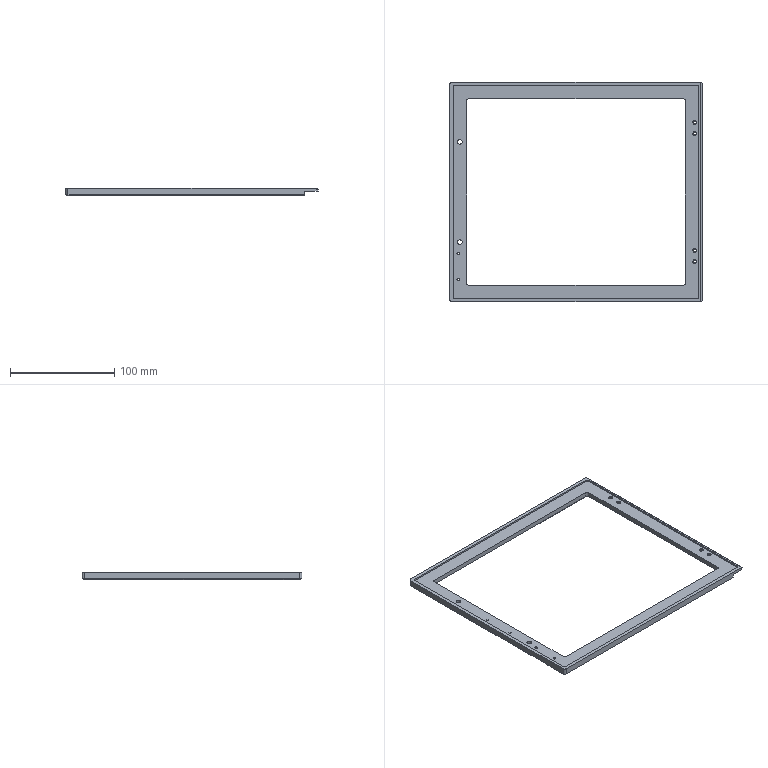NC program | NX | posted with a generic post | part box 241.5 x 210.5 x 7 mm
Whole program:
N10 G17 G21 G94 G90
(FLOOR_WALL_COPY , TOOL : D10)
N12 T10 M6
N14 G54
N16 G17 G0 G90 X128.75 Y-105.247 S9500 M3
N18 G43 Z75. H10
N20 Z5.033
N22 G94 G1 Z2.033 F800.
N24 X125.75
N26 X-125.75 F3000.
N28 Y-97.305
N30 X125.75
N32 Y-89.363
N34 X-125.75
N36 Y-81.42
N38 X-104.75
N40 Y-73.478
N42 X-125.75
N44 Y-65.536
N46 X-104.75
N48 Y-57.594
N50 X-125.75
N52 Y-49.652
N54 X-104.75
N56 Y-41.709
N58 X-125.75
N60 Y-33.767
N62 X-104.75
N64 Y-25.825
N66 X-125.75
N68 Y-17.883
N70 X-104.75
N72 Y-9.941
N74 X-125.75
N76 Y-1.999
N78 X-104.75
N80 Y5.944
N82 X-125.75
N84 Y13.886
N86 X-104.75
N88 Y21.828
N90 X-125.75
N92 Y29.77
N94 X-104.75
N96 Y37.712
N98 X-125.75
N100 Y45.655
N102 X-104.75
N104 Y53.597
N106 X-125.75
N108 Y61.539
N110 X-104.75
N112 Y69.481
N114 X-125.75
N116 Y77.423
N118 X-104.75
N120 Y85.366
N122 X-125.75
N124 X-128.75
N126 Z5.033
N128 G0 Z75.
N130 X104.75 Y-66.617
N132 Z6.
N134 G1 Y-81.42 Z2.033 F800.
N136 X125.75 F3000.
N138 Y-73.478
N140 X104.75
N142 Y-65.536
N144 X125.75
N146 Y-57.594
N148 X104.75
N150 Y-49.652
N152 X125.75
N154 Y-41.709
N156 X104.75
N158 Y-33.767
N160 X125.75
N162 Y-25.825
N164 X104.75
N166 Y-17.883
N168 X125.75
N170 Y-9.941
N172 X104.75
N174 Y-1.999
N176 X125.75
N178 Y5.944
N180 X104.75
N182 Y13.886
N184 X125.75
N186 Y21.828
N188 X104.75
N190 Y29.77
N192 X125.75
N194 Y37.712
N196 X104.75
N198 Y45.655
N200 X125.75
N202 Y53.597
N204 X104.75
N206 Y61.539
N208 X125.75
N210 Y69.481
N212 X104.75
N214 Y77.423
N216 X125.75
N218 Y85.366
N220 X104.75
N222 X101.75
N224 Z5.033
N226 G0 Z75.
N228 X-128.75 Y93.308
N230 Z5.033
N232 G1 Z2.033 F800.
N234 X-125.75
N236 X125.75 F3000.
N238 Y101.25
N240 X-125.75
N242 X-128.75
N244 Z5.033
N246 G0 Z75.
N248 X128.75 Y-105.247
N250 Z4.067
N252 G1 Z1.067 F800.
N254 X125.75
N256 X-125.75 F3000.
N258 Y-97.305
N260 X125.75
N262 Y-89.363
N264 X-125.75
N266 Y-81.42
N268 X-104.75
N270 Y-73.478
N272 X-125.75
N274 Y-65.536
N276 X-104.75
N278 Y-57.594
N280 X-125.75
N282 Y-49.652
N284 X-104.75
N286 Y-41.709
N288 X-125.75
N290 Y-33.767
N292 X-104.75
N294 Y-25.825
N296 X-125.75
N298 Y-17.883
N300 X-104.75
N302 Y-9.941
N304 X-125.75
N306 Y-1.999
N308 X-104.75
N310 Y5.944
N312 X-125.75
N314 Y13.886
N316 X-104.75
N318 Y21.828
N320 X-125.75
N322 Y29.77
N324 X-104.75
N326 Y37.712
N328 X-125.75
N330 Y45.655
N332 X-104.75
N334 Y53.597
N336 X-125.75
N338 Y61.539
N340 X-104.75
N342 Y69.481
N344 X-125.75
N346 Y77.423
N348 X-104.75
N350 Y85.366
N352 X-125.75
N354 X-128.75
N356 Z4.067
N358 G0 Z75.
N360 X104.75 Y-66.617
N362 Z5.033
N364 G1 Y-81.42 Z1.067 F800.
N366 X125.75 F3000.
N368 Y-73.478
N370 X104.75
N372 Y-65.536
N374 X125.75
N376 Y-57.594
N378 X104.75
N380 Y-49.652
N382 X125.75
N384 Y-41.709
N386 X104.75
N388 Y-33.767
N390 X125.75
N392 Y-25.825
N394 X104.75
N396 Y-17.883
N398 X125.75
N400 Y-9.941
N402 X104.75
N404 Y-1.999
N406 X125.75
N408 Y5.944
N410 X104.75
N412 Y13.886
N414 X125.75
N416 Y21.828
N418 X104.75
N420 Y29.77
N422 X125.75
N424 Y37.712
N426 X104.75
N428 Y45.655
N430 X125.75
N432 Y53.597
N434 X104.75
N436 Y61.539
N438 X125.75
N440 Y69.481
N442 X104.75
N444 Y77.423
N446 X125.75
N448 Y85.366
N450 X104.75
N452 X101.75
N454 Z4.067
N456 G0 Z75.
N458 X-128.75 Y93.308
N460 Z4.067
N462 G1 Z1.067 F800.
N464 X-125.75
N466 X125.75 F3000.
N468 Y101.25
N470 X-125.75
N472 X-128.75
N474 Z4.067
N476 G0 Z75.
N478 X128.75 Y-105.247
N480 Z3.1
N482 G1 Z0.1 F800.
N484 X125.75
N486 X-125.75 F3000.
N488 Y-97.305
N490 X125.75
N492 Y-89.363
N494 X-125.75
N496 Y-81.42
N498 X-104.75
N500 Y-73.478
N502 X-125.75
N504 Y-65.536
N506 X-104.75
N508 Y-57.594
N510 X-125.75
N512 Y-49.652
N514 X-104.75
N516 Y-41.709
N518 X-125.75
N520 Y-33.767
N522 X-104.75
N524 Y-25.825
N526 X-125.75
N528 Y-17.883
N530 X-104.75
N532 Y-9.941
N534 X-125.75
N536 Y-1.999
N538 X-104.75
N540 Y5.944
N542 X-125.75
N544 Y13.886
N546 X-104.75
N548 Y21.828
N550 X-125.75
N552 Y29.77
N554 X-104.75
N556 Y37.712
N558 X-125.75
N560 Y45.655
N562 X-104.75
N564 Y53.597
N566 X-125.75
N568 Y61.539
N570 X-104.75
N572 Y69.481
N574 X-125.75
N576 Y77.423
N578 X-104.75
N580 Y85.366
N582 X-125.75
N584 X-128.75
N586 Z3.1
N588 G0 Z75.
N590 X104.75 Y-66.617
N592 Z4.067
N594 G1 Y-81.42 Z0.1 F800.
N596 X125.75 F3000.
N598 Y-73.478
N600 X104.75
N602 Y-65.536
N604 X125.75
N606 Y-57.594
N608 X104.75
N610 Y-49.652
N612 X125.75
N614 Y-41.709
N616 X104.75
N618 Y-33.767
N620 X125.75
N622 Y-25.825
N624 X104.75
N626 Y-17.883
N628 X125.75
N630 Y-9.941
N632 X104.75
N634 Y-1.999
N636 X125.75
N638 Y5.944
N640 X104.75
N642 Y13.886
N644 X125.75
N646 Y21.828
N648 X104.75
N650 Y29.77
N652 X125.75
N654 Y37.712
N656 X104.75
N658 Y45.655
N660 X125.75
N662 Y53.597
N664 X104.75
N666 Y61.539
N668 X125.75
N670 Y69.481
N672 X104.75
N674 Y77.423
N676 X125.75
N678 Y85.366
N680 X104.75
N682 X101.75
N684 Z3.1
N686 G0 Z75.
N688 X-128.75 Y93.308
N690 Z3.1
N692 G1 Z0.1 F800.
N694 X-125.75
N696 X125.75 F3000.
N698 Y101.25
N700 X-125.75
N702 X-128.75
N704 Z3.1
N706 G0 Z75.
(FLOOR_WALL_COPY_COPY , TOOL : D10)
N708 X128.75 Y-105.247
N710 Z3.
N712 G1 Z0. F800.
N714 X125.75
N716 X-125.75 F1400.
N718 Y-97.305
N720 X125.75
N722 Y-89.363
N724 X-125.75
N726 Y-81.42
N728 X-104.75
N730 Y-73.478
N732 X-125.75
N734 Y-65.536
N736 X-104.75
N738 Y-57.594
N740 X-125.75
N742 Y-49.652
N744 X-104.75
N746 Y-41.709
N748 X-125.75
N750 Y-33.767
N752 X-104.75
N754 Y-25.825
N756 X-125.75
N758 Y-17.883
N760 X-104.75
N762 Y-9.941
N764 X-125.75
N766 Y-1.999
N768 X-104.75
N770 Y5.944
N772 X-125.75
N774 Y13.886
N776 X-104.75
N778 Y21.828
N780 X-125.75
N782 Y29.77
N784 X-104.75
N786 Y37.712
N788 X-125.75
N790 Y45.655
N792 X-104.75
N794 Y53.597
N796 X-125.75
N798 Y61.539
N800 X-104.75
N802 Y69.481
N804 X-125.75
N806 Y77.423
N808 X-104.75
N810 Y85.366
N812 X-125.75
N814 X-128.75
N816 Z3.
N818 G0 Z75.
N820 X104.75 Y-59.029
N822 Z6.
N824 G1 Y-81.42 Z0. F800.
N826 X125.75 F1400.
N828 Y-73.478
N830 X104.75
N832 Y-65.536
N834 X125.75
N836 Y-57.594
N838 X104.75
N840 Y-49.652
N842 X125.75
N844 Y-41.709
N846 X104.75
N848 Y-33.767
N850 X125.75
N852 Y-25.825
N854 X104.75
N856 Y-17.883
N858 X125.75
N860 Y-9.941
N862 X104.75
N864 Y-1.999
N866 X125.75
N868 Y5.944
N870 X104.75
N872 Y13.886
N874 X125.75
N876 Y21.828
N878 X104.75
N880 Y29.77
N882 X125.75
N884 Y37.712
N886 X104.75
N888 Y45.655
N890 X125.75
N892 Y53.597
N894 X104.75
N896 Y61.539
N898 X125.75
N900 Y69.481
N902 X104.75
N904 Y77.423
N906 X125.75
N908 Y85.366
N910 X104.75
N912 X101.75
N914 Z3.
N916 G0 Z75.
N918 X-128.75 Y93.308
N920 Z3.
N922 G1 Z0. F800.
N924 X-125.75
N926 X125.75 F1400.
N928 Y101.25
N930 X-125.75
N932 X-128.75
N934 Z3.
N936 G0 Z75.
N938 M5
(FLOOR_WALL_2 , TOOL : D6)
N940 T06 M6
N942 G54
N944 G17 G0 G90 X-114.75 Y73.689 S9500 M3
N946 G43 Z75. H6
N948 Z1.1
N950 G94 G1 Y68.092 Z0.807 F1000.
N952 X-114.194 Y67.604 Z0.768
N954 X-113.102 Y66.237 Z0.676
N956 X-112.75 Y65.587 Z0.637
N958 X-112.398 Y66.237 Z0.599
N960 X-111.306 Y67.604 Z0.507
N962 X-110.75 Y68.092 Z0.468
N964 Y74.408 Z0.137
N966 X-111.306 Y74.896 Z0.098
N968 X-112.398 Y76.263 Z0.007
N970 X-112.75 Y76.913 Z-0.032
N972 X-113.102 Y76.263 Z-0.071
N974 X-114.194 Y74.896 Z-0.162
N976 X-114.75 Y74.408 Z-0.201
N978 Y71.25 Z-0.367
N980 Y68.092 F2500.
N982 G2 X-112.75 Y65.587 R9.1
N984 X-110.75 Y68.092 R9.1
N986 G1 Y74.408
N988 G2 X-112.75 Y76.913 R9.1
N990 X-114.75 Y74.408 R9.1
N992 G1 Y71.25
N994 X-117.75
N996 Y66.561
N998 G2 X-114.65 Y61.25 R6.1
N1000 G3 X-112.75 Y59.35 R1.9
N1002 X-110.85 Y61.25 R1.9
N1004 G2 X-107.75 Y66.561 R6.1
N1006 G1 Y75.939
N1008 G2 X-110.85 Y81.25 R6.1
N1010 G3 X-112.75 Y83.15 R1.9
N1012 X-114.65 Y81.25 R1.9
N1014 G2 X-117.75 Y75.939 R6.1
N1016 G1 Y71.25
N1018 X-120.75
N1020 Y64.35
N1022 G2 X-117.65 Y61.25 R3.1
N1024 G3 X-112.75 Y56.35 R4.9
N1026 X-107.85 Y61.25 R4.9
N1028 G2 X-104.75 Y64.35 R3.1
N1030 G1 Y78.15
N1032 G2 X-107.85 Y81.25 R3.1
N1034 G3 X-112.75 Y86.15 R4.9
N1036 X-117.65 Y81.25 R4.9
N1038 G2 X-120.75 Y78.15 R3.1
N1040 G1 Y71.25
N1042 Z0.633
N1044 G0 X-114.75 Y73.689
N1046 G1 Y68.092 Z0.34 F1000.
N1048 X-114.194 Y67.604 Z0.301
N1050 X-113.102 Y66.237 Z0.21
N1052 X-112.75 Y65.587 Z0.171
N1054 X-112.398 Y66.237 Z0.132
N1056 X-111.306 Y67.604 Z0.04
N1058 X-110.75 Y68.092 Z0.002
N1060 Y74.408 Z-0.329
N1062 X-111.306 Y74.896 Z-0.368
N1064 X-112.398 Y76.263 Z-0.46
N1066 X-112.75 Y76.913 Z-0.499
N1068 X-113.102 Y76.263 Z-0.537
N1070 X-114.194 Y74.896 Z-0.629
N1072 X-114.75 Y74.408 Z-0.668
N1074 Y71.25 Z-0.833
N1076 Y68.092 F2500.
N1078 G2 X-112.75 Y65.587 R9.1
N1080 X-110.75 Y68.092 R9.1
N1082 G1 Y74.408
N1084 G2 X-112.75 Y76.913 R9.1
N1086 X-114.75 Y74.408 R9.1
N1088 G1 Y71.25
N1090 X-117.75
N1092 Y66.561
N1094 G2 X-114.65 Y61.25 R6.1
N1096 G3 X-112.75 Y59.35 R1.9
N1098 X-110.85 Y61.25 R1.9
N1100 G2 X-107.75 Y66.561 R6.1
N1102 G1 Y75.939
N1104 G2 X-110.85 Y81.25 R6.1
N1106 G3 X-112.75 Y83.15 R1.9
N1108 X-114.65 Y81.25 R1.9
N1110 G2 X-117.75 Y75.939 R6.1
N1112 G1 Y71.25
N1114 X-120.75
N1116 Y64.35
N1118 G2 X-117.65 Y61.25 R3.1
N1120 G3 X-112.75 Y56.35 R4.9
N1122 X-107.85 Y61.25 R4.9
N1124 G2 X-104.75 Y64.35 R3.1
N1126 G1 Y78.15
N1128 G2 X-107.85 Y81.25 R3.1
N1130 G3 X-112.75 Y86.15 R4.9
N1132 X-117.65 Y81.25 R4.9
N1134 G2 X-120.75 Y78.15 R3.1
N1136 G1 Y71.25
N1138 Z0.167
N1140 G0 X-114.75 Y73.689
N1142 G1 Y68.092 Z-0.127 F1000.
N1144 X-114.194 Y67.604 Z-0.165
N1146 X-113.102 Y66.237 Z-0.257
N1148 X-112.75 Y65.587 Z-0.296
N1150 X-112.398 Y66.237 Z-0.335
N1152 X-111.306 Y67.604 Z-0.426
N1154 X-110.75 Y68.092 Z-0.465
N1156 Y74.408 Z-0.796
N1158 X-111.306 Y74.896 Z-0.835
N1160 X-112.398 Y76.263 Z-0.927
N1162 X-112.75 Y76.913 Z-0.965
N1164 X-113.102 Y76.263 Z-1.004
N1166 X-114.194 Y74.896 Z-1.096
N1168 X-114.75 Y74.408 Z-1.134
N1170 Y71.25 Z-1.3
N1172 Y68.092 F2500.
N1174 G2 X-112.75 Y65.587 R9.1
N1176 X-110.75 Y68.092 R9.1
N1178 G1 Y74.408
N1180 G2 X-112.75 Y76.913 R9.1
N1182 X-114.75 Y74.408 R9.1
N1184 G1 Y71.25
N1186 X-117.75
N1188 Y66.561
N1190 G2 X-114.65 Y61.25 R6.1
N1192 G3 X-112.75 Y59.35 R1.9
N1194 X-110.85 Y61.25 R1.9
N1196 G2 X-107.75 Y66.561 R6.1
N1198 G1 Y75.939
N1200 G2 X-110.85 Y81.25 R6.1
N1202 G3 X-112.75 Y83.15 R1.9
N1204 X-114.65 Y81.25 R1.9
N1206 G2 X-117.75 Y75.939 R6.1
N1208 G1 Y71.25
N1210 X-120.75
N1212 Y64.35
N1214 G2 X-117.65 Y61.25 R3.1
N1216 G3 X-112.75 Y56.35 R4.9
N1218 X-107.85 Y61.25 R4.9
N1220 G2 X-104.75 Y64.35 R3.1
N1222 G1 Y78.15
N1224 G2 X-107.85 Y81.25 R3.1
N1226 G3 X-112.75 Y86.15 R4.9
N1228 X-117.65 Y81.25 R4.9
N1230 G2 X-120.75 Y78.15 R3.1
N1232 G1 Y71.25
N1234 Z-0.3
N1236 G0 Z75.
N1238 X-111.85 Y16.614
N1240 Z1.
N1242 G1 Y25.4 Z0.54 F1000.
N1244 X-113.65 Z0.445
N1246 Y8. Z-0.467
N1248 Y-9.4 F2500.
N1250 X-111.85
N1252 Y25.4
N1254 X-113.65
N1256 Y8.
N1258 X-116.65
N1260 Y-12.4
N1262 X-108.85
N1264 Y28.4
N1266 X-116.65
N1268 Y8.
N1270 Z0.533
N1272 G0 X-111.85 Y16.614
N1274 G1 Y25.4 Z0.073 F1000.
N1276 X-113.65 Z-0.021
N1278 Y8. Z-0.933
N1280 Y-9.4 F2500.
N1282 X-111.85
N1284 Y25.4
N1286 X-113.65
N1288 Y8.
N1290 X-116.65
N1292 Y-12.4
N1294 X-108.85
N1296 Y28.4
N1298 X-116.65
N1300 Y8.
N1302 Z0.067
N1304 G0 X-111.85 Y16.614
N1306 G1 Y25.4 Z-0.394 F1000.
N1308 X-113.65 Z-0.488
N1310 Y8. Z-1.4
N1312 Y-9.4 F2500.
N1314 X-111.85
N1316 Y25.4
N1318 X-113.65
N1320 Y8.
N1322 X-116.65
N1324 Y-12.4
N1326 X-108.85
N1328 Y28.4
N1330 X-116.65
N1332 Y8.
N1334 Z-0.4
N1336 G0 Z75.
(FLOOR_WALL_4 , TOOL : D6)
N1338 X-109.053 Y24.095
N1340 Z-0.4
N1342 G1 Y28.2 Z-1.5 F1250.
N1344 Y-12.2
N1346 X-111.519
N1348 Y28.2
N1350 X-113.984
N1352 Y-12.2
N1354 X-116.45
N1356 Y28.2
N1358 Y27.5
N1360 Y28.5
N1362 X-116.75
N1364 Y-12.5
N1366 X-108.75
N1368 Y28.5
N1370 X-116.45
N1372 Y27.5
N1374 X-115.75
N1376 Z-0.5
N1378 G0 Z75.
N1380 X120.747 Y108.908
N1382 Z-3.4
N1384 G1 Z-4.4
N1386 Y107.834
N1388 Y-107.834
N1390 G2 X118.75 Y-108.25 R5.
N1392 G1 X118.29
N1394 Y108.25
N1396 X115.833
N1398 Y-108.25
N1400 X113.376
N1402 Y108.25
N1404 X111.05
N1406 Y73.15
N1408 G2 X110.918 Y72.227 R3.3
N1410 G1 Z-3.4
N1412 G0 Z75.
N1414 Z-3.4
N1416 G1 Z-4.4
N1418 G2 X111.099 Y71.151 R3.3
N1420 G1 Y51.849
N1422 G2 X110.918 Y50.773 R3.3
N1424 G1 Z-3.4
N1426 G0 Z75.
N1428 Z-3.4
N1430 G1 Z-4.4
N1432 G2 X111.05 Y49.85 R3.3
N1434 G1 Y-49.85
N1436 G2 X110.918 Y-50.773 R3.3
N1438 G1 Z-3.4
N1440 G0 Z75.
N1442 Z-3.4
N1444 G1 Z-4.4
N1446 G2 X111.099 Y-51.849 R3.3
N1448 G1 Y-71.151
N1450 G2 X110.918 Y-72.227 R3.3
N1452 G1 Z-3.4
N1454 G0 Z75.
N1456 X110.75 Y109.25
N1458 Z-3.4
N1460 G1 Z-4.4
N1462 Y108.25
N1464 Y73.15
N1466 G2 X110.602 Y72.219 R3.
N1468 X110.799 Y71.151 R3.
N1470 G1 Y51.849
N1472 G2 X110.602 Y50.781 R3.
N1474 X110.75 Y49.85 R3.
N1476 G1 Y-49.85
N1478 G2 X110.602 Y-50.781 R3.
N1480 X110.799 Y-51.849 R3.
N1482 G1 Y-71.151
N1484 G2 X110.602 Y-72.219 R3.
N1486 X110.75 Y-73.15 R3.
N1488 G1 Y-108.25
N1490 Y-109.25
N1492 Z-3.4
N1494 G0 Z75.
(FLOOR_WALL_4_COPY , TOOL : D6)
N1496 X-113.88 Y74.98
N1498 Z-0.3
N1500 G1 X-114.179 Y74.627 Z-0.424
N1502 X-114.75 Y74.144 Z-0.624
N1504 Y71.25 Z-1.4
N1506 Y68.356
N1508 G2 X-112.75 Y65.992 R9.3
N1510 X-110.75 Y68.356 R9.3
N1512 G1 Y74.144
N1514 G2 X-112.75 Y76.508 R9.3
N1516 X-114.75 Y74.144 R9.3
N1518 G1 Y71.25
N1520 X-117.75
N1522 Y66.79
N1524 G2 X-114.45 Y61.25 R6.3
N1526 G3 X-112.75 Y59.55 R1.7
N1528 X-111.05 Y61.25 R1.7
N1530 G2 X-107.75 Y66.79 R6.3
N1532 G1 Y75.71
N1534 G2 X-111.05 Y81.25 R6.3
N1536 G3 X-112.75 Y82.95 R1.7
N1538 X-114.45 Y81.25 R1.7
N1540 G2 X-117.75 Y75.71 R6.3
N1542 G1 Y71.25
N1544 X-120.75
N1546 Y64.55
N1548 G2 X-117.45 Y61.25 R3.3
N1550 G3 X-112.75 Y56.55 R4.7
N1552 X-108.05 Y61.25 R4.7
N1554 G2 X-104.75 Y64.55 R3.3
N1556 G1 Y77.95
N1558 G2 X-108.05 Y81.25 R3.3
N1560 G3 X-112.75 Y85.95 R4.7
N1562 X-117.45 Y81.25 R4.7
N1564 G2 X-120.75 Y77.95 R3.3
N1566 G1 Y71.25
N1568 G2 X-121.05 Y70.73 R0.6
N1570 G1 X-123.87
N1572 Z-0.4
N1574 G0 Z75.
N1576 X-120.63 Y64.668
N1578 Z-0.4
N1580 G1 Z-1.4
N1582 X-121.27 Y64.55
N1584 G3 X-120.75 Y64.25 R0.6
N1586 G2 X-117.75 Y61.25 R3.
N1588 G3 X-112.75 Y56.25 R5.
N1590 X-107.75 Y61.25 R5.
N1592 G2 X-104.75 Y64.25 R3.
N1594 G3 X-104.23 Y64.55 R0.6
N1596 G1 X-104.87 Y64.668
N1598 Z-0.4
N1600 G0 Z75.
N1602 Y77.832
N1604 Z-0.4
N1606 G1 Z-1.4
N1608 X-104.23 Y77.95
N1610 G3 X-104.75 Y78.25 R0.6
N1612 G2 X-107.75 Y81.25 R3.
N1614 G3 X-112.75 Y86.25 R5.
N1616 X-117.75 Y81.25 R5.
N1618 G2 X-120.75 Y78.25 R3.
N1620 G3 X-121.27 Y77.95 R0.6
N1622 G1 X-120.63 Y77.832
N1624 Z-0.4
N1626 G0 Z75.
N1628 M5
(CAVITY_MILL_COPY , TOOL : D2)
N1630 T02 M6
N1632 G54
N1634 G17 G0 G90 X109.199 Y-70.396 S9500 M3
N1636 G43 Z75. H2
N1638 Z-0.13
N1640 G94 G3 X108.797 Y-71.175 R1. F1000.
N1642 G1 Y-71.183 F1100.
N1644 G2 X108.306 Y-72.011 R0.995
N1646 X107.907 Y-72.162 R1.295
N1648 G1 X107.949 Y-72.17
N1650 G2 X108.75 Y-73.175 R1.
N1652 G3 X109.15 Y-73.975 R1.
N1654 G0 X109.199 Y-70.396 Z-0.326
N1656 G3 X108.797 Y-71.175 R1. F1000.
N1658 G1 Y-71.182 F1100.
N1660 G2 X108.306 Y-72.011 R0.995
N1662 X107.907 Y-72.162 R1.297
N1664 G1 X107.91 Y-72.164
N1666 X107.949 Y-72.17
N1668 G2 X108.75 Y-73.175 R1.
N1670 G3 X109.15 Y-73.975 R1.
N1672 G0 X109.199 Y-70.396 Z-0.522
N1674 G3 X108.797 Y-71.175 R1. F1000.
N1676 G1 Y-71.181 F1100.
N1678 G2 X108.306 Y-72.011 R0.995
N1680 X107.907 Y-72.162 R1.298
N1682 G1 X107.948 Y-72.17
N1684 G2 X108.75 Y-73.175 R1.
N1686 G3 X109.15 Y-73.975 R1.
N1688 G0 X109.199 Y-70.395 Z-0.717
N1690 G3 X108.797 Y-71.175 R1. F1000.
N1692 G1 Y-71.18 F1100.
N1694 G2 X108.306 Y-72.012 R0.995
N1696 X107.907 Y-72.162 R1.3
N1698 G1 X107.947 Y-72.17
N1700 G2 X108.75 Y-73.175 R1.
N1702 G3 X109.15 Y-73.975 R1.
N1704 G0 X109.199 Y-70.395 Z-0.913
N1706 G3 X108.797 Y-71.175 R1. F1000.
N1708 G1 Y-71.179 F1100.
N1710 G2 X108.306 Y-72.012 R0.995
N1712 X107.907 Y-72.162 R1.302
N1714 G1 X107.947 Y-72.17
N1716 G2 X108.75 Y-73.175 R1.
N1718 G3 X109.15 Y-73.975 R1.
N1720 G0 X109.199 Y-70.395 Z-1.109
N1722 G3 X108.797 Y-71.175 R1. F1000.
N1724 G1 Y-71.179 F1100.
N1726 G2 X108.306 Y-72.012 R0.995
N1728 X107.907 Y-72.162 R1.303
N1730 G1 X107.946 Y-72.169
N1732 G2 X108.75 Y-73.175 R1.
N1734 G3 X109.15 Y-73.975 R1.
N1736 G0 X109.199 Y-70.395 Z-1.304
N1738 G3 X108.797 Y-71.175 R1. F1000.
N1740 G1 Y-71.178 F1100.
N1742 G2 X108.306 Y-72.012 R0.995
N1744 X107.907 Y-72.162 R1.305
N1746 G1 X107.945 Y-72.169
N1748 G2 X108.75 Y-73.175 R1.
N1750 G3 X109.15 Y-73.975 R1.
N1752 G0 X109.199 Y-70.395 Z-1.5
N1754 G3 X108.797 Y-71.175 R1. F1000.
N1756 G1 Y-71.177 F1100.
N1758 G2 X108.306 Y-72.012 R0.994
N1760 X107.907 Y-72.162 R1.307
N1762 G1 X107.945 Y-72.169
N1764 G2 X108.75 Y-73.175 R1.
N1766 G3 X109.15 Y-73.975 R1.
N1768 G0 X109.199 Y-70.394 Z-1.693
N1770 G3 X108.797 Y-71.175 R1. F1000.
N1772 G2 X108.306 Y-72.012 R0.994 F1100.
N1774 X107.907 Y-72.162 R1.308
N1776 G1 X107.944 Y-72.169
N1778 G2 X108.75 Y-73.175 R1.
N1780 G3 X109.15 Y-73.975 R1.
N1782 G0 X109.199 Y-70.394 Z-1.887
N1784 G3 X108.797 Y-71.175 R1. F1000.
N1786 G2 X108.306 Y-72.012 R0.994 F1100.
N1788 X107.907 Y-72.162 R1.31
N1790 G1 X107.943 Y-72.169
N1792 G2 X108.75 Y-73.175 R1.
N1794 G3 X109.15 Y-73.975 R1.
N1796 G0 X109.199 Y-70.394 Z-2.08
N1798 G3 X108.797 Y-71.175 R1. F1000.
N1800 G2 X108.306 Y-72.012 R0.993 F1100.
N1802 X107.907 Y-72.162 R1.312
N1804 G1 X107.942 Y-72.169
N1806 G2 X108.75 Y-73.175 R1.
N1808 G3 X109.15 Y-73.975 R1.
N1810 G0 X109.199 Y-70.396 Z-2.273
N1812 G3 X108.797 Y-71.175 R1. F1000.
N1814 G2 X108.306 Y-72.012 R0.996 F1100.
N1816 X107.907 Y-72.162 R1.313
N1818 G1 X107.941 Y-72.168
N1820 G2 X108.75 Y-73.176 R1.
N1822 G3 X109.15 Y-73.976 R1.
N1824 G0 X109.199 Y-70.396 Z-2.467
N1826 G3 X108.798 Y-71.175 R1. F1000.
N1828 G2 X108.306 Y-72.012 R0.997 F1100.
N1830 X107.907 Y-72.162 R1.315
N1832 G1 X107.941 Y-72.168
N1834 G2 X108.75 Y-73.176 R1.
N1836 G3 X109.15 Y-73.976 R1.
N1838 G0 X109.199 Y-70.396 Z-2.66
N1840 G3 X108.798 Y-71.175 R1. F1000.
N1842 G2 X108.306 Y-72.012 R0.997 F1100.
N1844 X107.907 Y-72.162 R1.317
N1846 G1 X107.94 Y-72.168
N1848 G2 X108.75 Y-73.176 R1.
N1850 G3 X109.15 Y-73.976 R1.
N1852 G0 X109.199 Y-70.397 Z-2.853
N1854 G3 X108.798 Y-71.175 R1. F1000.
N1856 G2 X108.306 Y-72.013 R0.998 F1100.
N1858 X107.907 Y-72.162 R1.318
N1860 G1 X107.939 Y-72.168
N1862 G2 X108.75 Y-73.176 R1.
N1864 G3 X109.15 Y-73.976 R1.
N1866 G0 X109.199 Y-70.397 Z-3.047
N1868 G3 X108.798 Y-71.175 R1. F1000.
N1870 G2 X108.306 Y-72.013 R0.998 F1100.
N1872 X107.907 Y-72.162 R1.32
N1874 G1 X107.938 Y-72.168
N1876 G2 X108.75 Y-73.176 R1.
N1878 G3 X109.15 Y-73.976 R1.
N1880 G0 X109.199 Y-70.397 Z-3.24
N1882 G3 X108.798 Y-71.175 R1. F1000.
N1884 G2 X108.306 Y-72.013 R0.998 F1100.
N1886 X107.907 Y-72.162 R1.322
N1888 G1 X107.936 Y-72.168
N1890 G2 X108.75 Y-73.176 R1.
N1892 G3 X109.15 Y-73.976 R1.
N1894 G0 X109.199 Y-70.398 Z-3.433
N1896 G3 X108.798 Y-71.175 R1. F1000.
N1898 G2 X108.306 Y-72.013 R0.999 F1100.
N1900 X107.907 Y-72.162 R1.324
N1902 G1 X107.935 Y-72.167
N1904 G2 X108.75 Y-73.176 R1.
N1906 G3 X109.15 Y-73.976 R1.
N1908 G0 X109.199 Y-70.398 Z-3.627
N1910 G3 X108.798 Y-71.175 R1. F1000.
N1912 G2 X108.306 Y-72.013 R0.999 F1100.
N1914 X107.907 Y-72.162 R1.325
N1916 G1 X107.934 Y-72.167
N1918 G2 X108.75 Y-73.176 R1.
N1920 G3 X109.15 Y-73.976 R1.
N1922 G0 X109.199 Y-70.398 Z-3.82
N1924 G3 X108.798 Y-71.175 R1. F1000.
N1926 G2 X108.306 Y-72.013 R0.999 F1100.
N1928 X107.907 Y-72.162 R1.327
N1930 G1 X107.932 Y-72.167
N1932 G2 X108.75 Y-73.176 R1.
N1934 G3 X109.15 Y-73.976 R1.
N1936 G0 X109.199 Y-70.398 Z-4.013
N1938 G3 X108.798 Y-71.175 R1. F1000.
N1940 G2 X108.306 Y-72.013 R0.999 F1100.
N1942 X107.907 Y-72.162 R1.329
N1944 G1 X107.93 Y-72.166
N1946 G2 X108.75 Y-73.176 R1.
N1948 G3 X109.15 Y-73.976 R1.
N1950 G0 X109.199 Y-70.398 Z-4.207
N1952 G3 X108.799 Y-71.175 R1. F1000.
N1954 G2 X108.306 Y-72.013 R0.999 F1100.
N1956 X107.91 Y-72.162 R1.331
N1958 G1 X107.93 Y-72.166
N1960 G2 X108.75 Y-73.176 R1.
N1962 G3 X109.15 Y-73.976 R1.
N1964 G0 X109.199 Y-70.398 Z-4.4
N1966 G3 X108.799 Y-71.175 R1. F1000.
N1968 G2 X108.306 Y-72.013 R0.999 F1100.
N1970 X107.91 Y-72.162 R1.333
N1972 G1 X107.93 Y-72.166
N1974 G2 X108.75 Y-73.176 R1.
N1976 G3 X109.15 Y-73.976 R1.
N1978 G0 Z75.
N1980 Y-48.966
N1982 Z-0.13
N1984 G3 X108.75 Y-49.766 R1. F1000.
N1986 G1 Y-49.85 F1100.
N1988 G2 X107.837 Y-50.846 R1.004
N1990 X108.798 Y-51.837 R1.012
N1992 G3 X109.199 Y-52.618 R1.
N1994 G0 X109.15 Y-48.966 Z-0.326
N1996 G3 X108.75 Y-49.766 R1. F1000.
N1998 G1 Y-49.85 F1100.
N2000 G2 X107.837 Y-50.846 R1.004
N2002 X108.798 Y-51.837 R1.011
N2004 G3 X109.199 Y-52.619 R1.
N2006 G0 X109.15 Y-48.966 Z-0.522
N2008 G3 X108.75 Y-49.766 R1. F1000.
N2010 G1 Y-49.85 F1100.
N2012 G2 X107.837 Y-50.846 R1.003
N2014 X108.798 Y-51.837 R1.011
N2016 G3 X109.199 Y-52.619 R1.
N2018 G0 X109.15 Y-48.966 Z-0.717
N2020 G3 X108.75 Y-49.766 R1. F1000.
N2022 G1 Y-49.85 F1100.
N2024 G2 X107.837 Y-50.846 R1.003
N2026 X108.798 Y-51.837 R1.011
N2028 G3 X109.199 Y-52.619 R1.
N2030 G0 X109.15 Y-48.966 Z-0.913
N2032 G3 X108.75 Y-49.766 R1. F1000.
N2034 G1 Y-49.85 F1100.
N2036 G2 X107.837 Y-50.846 R1.003
N2038 X108.798 Y-51.837 R1.011
N2040 G3 X109.199 Y-52.619 R1.
N2042 G0 X109.15 Y-48.966 Z-1.109
N2044 G3 X108.75 Y-49.766 R1. F1000.
N2046 G1 Y-49.85 F1100.
N2048 G2 X107.838 Y-50.846 R1.003
N2050 X108.798 Y-51.837 R1.011
N2052 G3 X109.199 Y-52.62 R1.
N2054 G0 X109.15 Y-48.966 Z-1.304
N2056 G3 X108.75 Y-49.766 R1. F1000.
N2058 G1 Y-49.85 F1100.
N2060 G2 X107.838 Y-50.846 R1.003
N2062 X108.798 Y-51.837 R1.01
N2064 G3 X109.199 Y-52.62 R1.
N2066 G0 X109.15 Y-48.965 Z-1.5
N2068 G3 X108.75 Y-49.765 R1. F1000.
N2070 G1 Y-49.85 F1100.
N2072 G2 X107.838 Y-50.846 R1.002
N2074 X108.799 Y-51.837 R1.01
N2076 G3 X109.199 Y-52.62 R1.
N2078 G0 X109.15 Y-48.965 Z-1.693
N2080 G3 X108.75 Y-49.765 R1. F1000.
N2082 G1 Y-49.85 F1100.
N2084 G2 X107.838 Y-50.846 R1.002
N2086 X108.799 Y-51.837 R1.01
N2088 G3 X109.199 Y-52.621 R1.
N2090 G0 X109.15 Y-48.965 Z-1.887
N2092 G3 X108.75 Y-49.765 R1. F1000.
N2094 G1 Y-49.85 F1100.
N2096 G2 X107.838 Y-50.846 R1.002
N2098 X108.799 Y-51.837 R1.01
N2100 G3 X109.199 Y-52.621 R1.
N2102 G0 X109.15 Y-48.965 Z-2.08
N2104 G3 X108.75 Y-49.765 R1. F1000.
N2106 G1 Y-49.85 F1100.
N2108 G2 X107.838 Y-50.846 R1.002
N2110 X108.799 Y-51.838 R1.009
N2112 G3 X109.199 Y-52.621 R1.
N2114 G0 X109.15 Y-48.965 Z-2.273
N2116 G3 X108.75 Y-49.765 R1. F1000.
N2118 G1 Y-49.85 F1100.
N2120 G2 X107.838 Y-50.846 R1.001
N2122 X108.799 Y-51.838 R1.009
N2124 G3 X109.199 Y-52.621 R1.
N2126 G0 X109.15 Y-48.965 Z-2.467
N2128 G3 X108.75 Y-49.765 R1. F1000.
N2130 G1 Y-49.85 F1100.
N2132 G2 X107.838 Y-50.846 R1.001
N2134 X108.799 Y-51.838 R1.009
N2136 G3 X109.199 Y-52.622 R1.
N2138 G0 X109.15 Y-48.965 Z-2.66
N2140 G3 X108.75 Y-49.765 R1. F1000.
N2142 G1 Y-49.85 F1100.
N2144 G2 X107.838 Y-50.846 R1.001
N2146 X108.799 Y-51.838 R1.009
N2148 G3 X109.199 Y-52.622 R1.
N2150 G0 X109.15 Y-48.965 Z-2.853
N2152 G3 X108.75 Y-49.765 R1. F1000.
N2154 G1 Y-49.85 F1100.
N2156 G2 X107.838 Y-50.846 R1.001
N2158 X108.799 Y-51.838 R1.009
N2160 G3 X109.199 Y-52.622 R1.
N2162 G0 X109.15 Y-48.965 Z-3.047
N2164 G3 X108.75 Y-49.765 R1. F1000.
N2166 G1 Y-49.85 F1100.
N2168 G2 X107.838 Y-50.846 R1.
N2170 X108.799 Y-51.838 R1.008
N2172 G3 X109.199 Y-52.622 R1.
N2174 G0 X109.15 Y-48.965 Z-3.24
N2176 G3 X108.75 Y-49.765 R1. F1000.
N2178 G1 Y-49.85 F1100.
N2180 G2 X107.838 Y-50.846 R1.
N2182 X108.799 Y-51.838 R1.008
N2184 G3 X109.199 Y-52.623 R1.
N2186 G0 X109.15 Y-48.965 Z-3.433
N2188 G3 X108.75 Y-49.765 R1. F1000.
N2190 G1 Y-49.85 F1100.
N2192 G2 X107.839 Y-50.846 R1.
N2194 X108.799 Y-51.838 R1.008
N2196 G3 X109.199 Y-52.623 R1.
N2198 G0 X109.15 Y-48.964 Z-3.627
N2200 G3 X108.75 Y-49.764 R1. F1000.
N2202 G1 Y-49.85 F1100.
N2204 G2 X107.839 Y-50.846 R1.
N2206 X108.799 Y-51.838 R1.008
N2208 G3 X109.199 Y-52.623 R1.
N2210 G0 X109.15 Y-48.965 Z-3.82
N2212 G3 X108.75 Y-49.765 R1. F1000.
N2214 G1 Y-49.85 F1100.
N2216 G2 X107.839 Y-50.846 R1.
N2218 X108.799 Y-51.838 R1.008
N2220 G3 X109.199 Y-52.623 R1.
N2222 G0 X109.15 Y-48.964 Z-4.013
N2224 G3 X108.75 Y-49.764 R1. F1000.
N2226 G1 Y-49.85 F1100.
N2228 G2 X107.839 Y-50.846 R0.999
N2230 X108.799 Y-51.838 R1.007
N2232 G3 X109.199 Y-52.624 R1.
N2234 G0 X109.15 Y-48.964 Z-4.207
N2236 G3 X108.75 Y-49.764 R1. F1000.
N2238 G1 Y-49.85 F1100.
N2240 G2 X107.839 Y-50.846 R0.999
N2242 X108.799 Y-51.838 R1.007
N2244 G3 X109.199 Y-52.624 R1.
N2246 G0 X109.15 Y-48.964 Z-4.4
N2248 G3 X108.75 Y-49.764 R1. F1000.
N2250 G1 Y-49.85 F1100.
N2252 G2 X107.839 Y-50.846 R0.999
N2254 X108.799 Y-51.838 R1.007
N2256 G3 X109.199 Y-52.624 R1.
N2258 G0 Z75.
N2260 Y52.626
N2262 Z-0.13
N2264 G3 X108.799 Y51.841 R1. F1000.
N2266 G2 X107.837 Y50.846 R1.012 F1100.
N2268 X108.75 Y49.824 R1.004
N2270 G3 X109.15 Y49.024 R1.
N2272 G0 X109.199 Y52.626 Z-0.326
N2274 G3 X108.799 Y51.841 R1. F1000.
N2276 G2 X107.837 Y50.846 R1.012 F1100.
N2278 X108.75 Y49.824 R1.004
N2280 G3 X109.15 Y49.024 R1.
N2282 G0 X109.199 Y52.626 Z-0.522
N2284 G3 X108.799 Y51.841 R1. F1000.
N2286 G2 X107.837 Y50.846 R1.012 F1100.
N2288 X108.75 Y49.824 R1.004
N2290 G3 X109.15 Y49.024 R1.
N2292 G0 X109.199 Y52.627 Z-0.717
N2294 G3 X108.799 Y51.841 R1. F1000.
N2296 G2 X107.837 Y50.846 R1.012 F1100.
N2298 X108.75 Y49.824 R1.003
N2300 G3 X109.15 Y49.024 R1.
N2302 G0 X109.199 Y52.627 Z-0.913
N2304 G3 X108.799 Y51.841 R1. F1000.
N2306 G2 X107.837 Y50.846 R1.012 F1100.
N2308 X108.75 Y49.824 R1.003
N2310 G3 X109.15 Y49.024 R1.
N2312 G0 X109.199 Y52.627 Z-1.109
N2314 G3 X108.799 Y51.841 R1. F1000.
N2316 G2 X107.838 Y50.846 R1.011 F1100.
N2318 X108.75 Y49.824 R1.003
N2320 G3 X109.15 Y49.024 R1.
N2322 G0 X109.199 Y52.627 Z-1.304
N2324 G3 X108.799 Y51.841 R1. F1000.
N2326 G2 X107.838 Y50.846 R1.011 F1100.
N2328 X108.75 Y49.823 R1.003
N2330 G3 X109.15 Y49.023 R1.
N2332 G0 X109.199 Y52.627 Z-1.5
N2334 G3 X108.799 Y51.841 R1. F1000.
N2336 G2 X107.838 Y50.846 R1.011 F1100.
N2338 X108.75 Y49.823 R1.003
N2340 G3 X109.15 Y49.023 R1.
N2342 G0 X109.199 Y52.627 Z-1.693
N2344 G3 X108.799 Y51.841 R1. F1000.
N2346 G2 X107.838 Y50.846 R1.011 F1100.
N2348 X108.75 Y49.823 R1.002
N2350 G3 X109.15 Y49.023 R1.
N2352 G0 X109.199 Y52.627 Z-1.887
N2354 G3 X108.799 Y51.841 R1. F1000.
N2356 G2 X107.838 Y50.846 R1.011 F1100.
N2358 X108.75 Y49.823 R1.002
N2360 G3 X109.15 Y49.023 R1.
N2362 G0 X109.199 Y52.628 Z-2.08
N2364 G3 X108.799 Y51.841 R1. F1000.
N2366 G2 X107.838 Y50.846 R1.011 F1100.
N2368 X108.75 Y49.823 R1.002
N2370 G3 X109.15 Y49.023 R1.
N2372 G0 X109.199 Y52.628 Z-2.273
N2374 G3 X108.799 Y51.841 R1. F1000.
N2376 G2 X107.838 Y50.846 R1.011 F1100.
N2378 X108.75 Y49.823 R1.002
N2380 G3 X109.15 Y49.023 R1.
N2382 G0 X109.199 Y52.628 Z-2.467
N2384 G3 X108.799 Y51.841 R1. F1000.
N2386 G2 X107.838 Y50.846 R1.01 F1100.
N2388 X108.75 Y49.823 R1.002
N2390 G3 X109.15 Y49.023 R1.
N2392 G0 X109.199 Y52.628 Z-2.66
N2394 G3 X108.799 Y51.841 R1. F1000.
N2396 G2 X107.838 Y50.846 R1.01 F1100.
N2398 X108.75 Y49.823 R1.001
N2400 G3 X109.15 Y49.023 R1.
N2402 G0 X109.199 Y52.628 Z-2.853
N2404 G3 X108.799 Y51.842 R1. F1000.
N2406 G2 X107.838 Y50.846 R1.01 F1100.
N2408 X108.75 Y49.823 R1.001
N2410 G3 X109.15 Y49.023 R1.
N2412 G0 X109.199 Y52.628 Z-3.047
N2414 G3 X108.799 Y51.842 R1. F1000.
N2416 G2 X107.838 Y50.846 R1.01 F1100.
N2418 X108.75 Y49.823 R1.001
N2420 G3 X109.15 Y49.023 R1.
N2422 G0 X109.199 Y52.628 Z-3.24
N2424 G3 X108.799 Y51.842 R1. F1000.
N2426 G2 X107.838 Y50.846 R1.01 F1100.
N2428 X108.75 Y49.823 R1.001
N2430 G3 X109.15 Y49.023 R1.
N2432 G0 X109.199 Y52.629 Z-3.433
N2434 G3 X108.799 Y51.842 R1. F1000.
N2436 G2 X107.839 Y50.846 R1.01 F1100.
N2438 X108.749 Y49.878 R1.
N2440 G1 X108.75 Y49.823
N2442 G3 X109.15 Y49.025 R1.
N2444 G0 X109.199 Y52.629 Z-3.627
N2446 G3 X108.799 Y51.842 R1. F1000.
N2448 G2 X107.839 Y50.846 R1.01 F1100.
N2450 X108.749 Y49.878 R0.999
N2452 G1 X108.75 Y49.823
N2454 G3 X109.15 Y49.025 R1.
N2456 G0 X109.199 Y52.629 Z-3.82
N2458 G3 X108.8 Y51.842 R1. F1000.
N2460 G2 X107.839 Y50.846 R1.01 F1100.
N2462 X108.75 Y49.878 R0.999
N2464 G1 Y49.823
N2466 G3 X109.15 Y49.025 R1.
N2468 G0 X109.199 Y52.629 Z-4.013
N2470 G3 X108.8 Y51.842 R1. F1000.
N2472 G2 X107.839 Y50.846 R1.009 F1100.
N2474 X108.75 Y49.878 R1.
N2476 G1 Y49.823
N2478 G3 X109.15 Y49.024 R1.
N2480 G0 X109.199 Y52.629 Z-4.207
N2482 G3 X108.8 Y51.842 R1. F1000.
N2484 G2 X107.839 Y50.846 R1.009 F1100.
N2486 X108.75 Y49.878 R0.999
N2488 G1 Y49.823
N2490 G3 X109.15 Y49.024 R1.
N2492 G0 X109.199 Y52.629 Z-4.4
N2494 G3 X108.8 Y51.842 R1. F1000.
N2496 G2 X107.839 Y50.846 R1.009 F1100.
N2498 X108.75 Y49.823 R0.999
N2500 G3 X109.15 Y49.023 R1.
N2502 G0 Z75.
N2504 Y73.986
N2506 Z-0.13
N2508 G3 X108.75 Y73.186 R1. F1000.
N2510 G1 Y73.15 F1100.
N2512 G2 X107.85 Y72.154 R1.007
N2514 G1 Y72.152
N2516 G2 X108.798 Y71.177 R1.004
N2518 G3 X109.199 Y70.405 R1.
N2520 G0 X109.15 Y73.986 Z-0.326
N2522 G3 X108.75 Y73.186 R1. F1000.
N2524 G1 Y73.15 F1100.
N2526 G2 X107.85 Y72.154 R1.006
N2528 G1 Y72.152
N2530 G2 X108.798 Y71.177 R1.004
N2532 G3 X109.199 Y70.404 R1.
N2534 G0 X109.15 Y73.986 Z-0.522
N2536 G3 X108.75 Y73.186 R1. F1000.
N2538 G1 Y73.15 F1100.
N2540 G2 X107.85 Y72.154 R1.006
N2542 G1 Y72.152
N2544 G2 X108.798 Y71.177 R1.004
N2546 G3 X109.199 Y70.404 R1.
N2548 G0 X109.15 Y73.986 Z-0.717
N2550 G3 X108.75 Y73.186 R1. F1000.
N2552 G1 Y73.15 F1100.
N2554 G2 X107.85 Y72.154 R1.006
N2556 G1 Y72.152
N2558 G2 X108.798 Y71.177 R1.004
N2560 G3 X109.199 Y70.404 R1.
N2562 G0 X109.15 Y73.986 Z-0.913
N2564 G3 X108.75 Y73.186 R1. F1000.
N2566 G1 Y73.15 F1100.
N2568 G2 X107.85 Y72.154 R1.006
N2570 G1 Y72.152
N2572 G2 X108.798 Y71.177 R1.004
N2574 G3 X109.199 Y70.403 R1.
N2576 G0 X109.15 Y73.986 Z-1.109
N2578 G3 X108.75 Y73.186 R1. F1000.
N2580 G1 Y73.15 F1100.
N2582 G2 X107.85 Y72.154 R1.006
N2584 G1 Y72.152
N2586 G2 X108.798 Y71.177 R1.005
N2588 G3 X109.199 Y70.403 R1.
N2590 G0 X109.15 Y73.986 Z-1.304
N2592 G3 X108.75 Y73.186 R1. F1000.
N2594 G1 Y73.15 F1100.
N2596 G2 X107.85 Y72.154 R1.005
N2598 G1 Y72.152
N2600 G2 X108.799 Y71.176 R1.005
N2602 G3 X109.199 Y70.403 R1.
N2604 G0 X109.15 Y73.986 Z-1.5
N2606 G3 X108.75 Y73.186 R1. F1000.
N2608 G1 Y73.15 F1100.
N2610 G2 X107.85 Y72.154 R1.005
N2612 G1 Y72.153
N2614 G2 X108.799 Y71.176 R1.005
N2616 G3 X109.199 Y70.402 R1.
N2618 G0 X109.15 Y73.987 Z-1.693
N2620 G3 X108.75 Y73.187 R1. F1000.
N2622 G1 Y73.15 F1100.
N2624 G2 X107.85 Y72.154 R1.005
N2626 G1 Y72.153
N2628 G2 X108.799 Y71.176 R1.005
N2630 G3 X109.199 Y70.402 R1.
N2632 G0 X109.15 Y73.987 Z-1.887
N2634 G3 X108.75 Y73.187 R1. F1000.
N2636 G1 Y73.15 F1100.
N2638 G2 X107.85 Y72.154 R1.005
N2640 X108.799 Y71.176 R1.005
N2642 G3 X109.199 Y70.402 R1.
N2644 G0 X109.15 Y73.987 Z-2.08
N2646 G3 X108.75 Y73.187 R1. F1000.
N2648 G1 Y73.15 F1100.
N2650 G2 X107.85 Y72.154 R1.005
N2652 X108.799 Y71.176 R1.005
N2654 G3 X109.199 Y70.401 R1.
N2656 G0 X109.15 Y73.987 Z-2.273
N2658 G3 X108.75 Y73.187 R1. F1000.
N2660 G1 Y73.15 F1100.
N2662 G2 X107.85 Y72.154 R1.005
N2664 X108.799 Y71.175 R1.005
N2666 G3 X109.199 Y70.401 R1.
N2668 G0 X109.15 Y73.987 Z-2.467
N2670 G3 X108.75 Y73.187 R1. F1000.
N2672 G1 Y73.15 F1100.
N2674 G2 X107.85 Y72.154 R1.004
N2676 X108.799 Y71.175 R1.005
N2678 G3 X109.199 Y70.401 R1.
N2680 G0 X109.15 Y73.987 Z-2.66
N2682 G3 X108.75 Y73.187 R1. F1000.
N2684 G1 Y73.15 F1100.
N2686 G2 X107.85 Y72.154 R1.004
N2688 X108.799 Y71.175 R1.006
N2690 G3 X109.199 Y70.4 R1.
N2692 G0 X109.15 Y73.987 Z-2.853
N2694 G3 X108.75 Y73.187 R1. F1000.
N2696 G1 Y73.15 F1100.
N2698 G2 X107.85 Y72.154 R1.004
N2700 X108.799 Y71.175 R1.006
N2702 G3 X109.199 Y70.4 R1.
N2704 G0 X109.15 Y73.987 Z-3.047
N2706 G3 X108.75 Y73.187 R1. F1000.
N2708 G1 Y73.152 F1100.
N2710 G2 X107.85 Y72.154 R1.004
N2712 X108.799 Y71.175 R1.006
N2714 G3 X109.199 Y70.4 R1.
N2716 G0 X109.15 Y73.987 Z-3.24
N2718 G3 X108.75 Y73.187 R1. F1000.
N2720 G1 Y73.152 F1100.
N2722 G2 X107.85 Y72.154 R1.004
N2724 X108.799 Y71.175 R1.006
N2726 G3 X109.199 Y70.399 R1.
N2728 G0 X109.15 Y73.988 Z-3.433
N2730 G3 X108.75 Y73.188 R1. F1000.
N2732 G1 Y73.152 F1100.
N2734 G2 X107.851 Y72.154 R1.004
N2736 X108.799 Y71.175 R1.006
N2738 G3 X109.199 Y70.399 R1.
N2740 G0 X109.15 Y73.988 Z-3.627
N2742 G3 X108.75 Y73.188 R1. F1000.
N2744 G1 Y73.152 F1100.
N2746 G2 X107.852 Y72.154 R1.004
N2748 X108.799 Y71.175 R1.006
N2750 G3 X109.199 Y70.399 R1.
N2752 G0 X109.15 Y73.988 Z-3.82
N2754 G3 X108.75 Y73.188 R1. F1000.
N2756 G1 Y73.151 F1100.
N2758 G2 X107.853 Y72.154 R1.003
N2760 X108.799 Y71.175 R1.006
N2762 G3 X109.199 Y70.4 R1.
N2764 G0 X109.15 Y73.988 Z-4.013
N2766 G3 X108.75 Y73.188 R1. F1000.
N2768 G1 Y73.151 F1100.
N2770 G2 X107.854 Y72.154 R1.003
N2772 X108.799 Y71.175 R1.006
N2774 G3 X109.199 Y70.4 R1.
N2776 G0 X109.15 Y73.988 Z-4.207
N2778 G3 X108.75 Y73.188 R1. F1000.
N2780 G1 Y73.151 F1100.
N2782 G2 X107.854 Y72.154 R1.003
N2784 X108.799 Y71.175 R1.006
N2786 G3 X109.199 Y70.4 R1.
N2788 G0 X109.15 Y73.988 Z-4.4
N2790 G3 X108.75 Y73.188 R1. F1000.
N2792 G1 Y73.151 F1100.
N2794 G2 X107.855 Y72.154 R1.003
N2796 X108.799 Y71.175 R1.006
N2798 G3 X109.199 Y70.4 R1.
N2800 G0 Z75.
N2802 X-107.15 Y27.484
N2804 Z-0.13
N2806 G3 X-106.75 Y28.284 R1. F1000.
N2808 G1 Y30.5 F1100.
N2810 X-108.966
N2812 G3 X-109.766 Y30.1 R1.
N2814 G0 X-107.15 Y27.484 Z-0.326
N2816 G3 X-106.75 Y28.284 R1. F1000.
N2818 G1 Y30.5 F1100.
N2820 X-108.966
N2822 G3 X-109.766 Y30.1 R1.
N2824 G0 X-107.15 Y27.484 Z-0.522
N2826 G3 X-106.75 Y28.284 R1. F1000.
N2828 G1 Y30.5 F1100.
N2830 X-108.966
N2832 G3 X-109.766 Y30.1 R1.
N2834 G0 X-107.15 Y27.484 Z-0.717
N2836 G3 X-106.75 Y28.284 R1. F1000.
N2838 G1 Y30.5 F1100.
N2840 X-108.966
N2842 G3 X-109.766 Y30.1 R1.
N2844 G0 X-107.15 Y27.484 Z-0.913
N2846 G3 X-106.75 Y28.284 R1. F1000.
N2848 G1 Y30.5 F1100.
N2850 X-108.966
N2852 G3 X-109.766 Y30.1 R1.
N2854 G0 X-107.15 Y27.484 Z-1.109
N2856 G3 X-106.75 Y28.284 R1. F1000.
N2858 G1 Y30.5 F1100.
N2860 X-108.966
N2862 G3 X-109.766 Y30.1 R1.
N2864 G0 X-107.15 Y27.484 Z-1.304
N2866 G3 X-106.75 Y28.284 R1. F1000.
N2868 G1 Y30.5 F1100.
N2870 X-108.966
N2872 G3 X-109.766 Y30.1 R1.
N2874 G0 X-107.15 Y27.484 Z-1.5
N2876 G3 X-106.75 Y28.284 R1. F1000.
N2878 G1 Y30.5 F1100.
N2880 X-108.966
N2882 G3 X-109.766 Y30.1 R1.
N2884 G0 Z75.
N2886 X-115.734
N2888 Z-0.13
N2890 G3 X-116.534 Y30.5 R1. F1000.
N2892 G1 X-118.75 F1100.
N2894 Y28.284
N2896 G3 X-118.35 Y27.484 R1.
N2898 G0 X-115.734 Y30.1 Z-0.326
N2900 G3 X-116.534 Y30.5 R1. F1000.
N2902 G1 X-118.75 F1100.
N2904 Y28.284
N2906 G3 X-118.35 Y27.484 R1.
N2908 G0 X-115.734 Y30.1 Z-0.522
N2910 G3 X-116.534 Y30.5 R1. F1000.
N2912 G1 X-118.75 F1100.
N2914 Y28.284
N2916 G3 X-118.35 Y27.484 R1.
N2918 G0 X-115.734 Y30.1 Z-0.717
N2920 G3 X-116.534 Y30.5 R1. F1000.
N2922 G1 X-118.75 F1100.
N2924 Y28.284
N2926 G3 X-118.35 Y27.484 R1.
N2928 G0 X-115.734 Y30.1 Z-0.913
N2930 G3 X-116.534 Y30.5 R1. F1000.
N2932 G1 X-118.75 F1100.
N2934 Y28.284
N2936 G3 X-118.35 Y27.484 R1.
N2938 G0 X-115.734 Y30.1 Z-1.109
N2940 G3 X-116.534 Y30.5 R1. F1000.
N2942 G1 X-118.75 F1100.
N2944 Y28.284
N2946 G3 X-118.35 Y27.484 R1.
N2948 G0 X-115.734 Y30.1 Z-1.304
N2950 G3 X-116.534 Y30.5 R1. F1000.
N2952 G1 X-118.75 F1100.
N2954 Y28.284
N2956 G3 X-118.35 Y27.484 R1.
N2958 G0 X-115.734 Y30.1 Z-1.5
N2960 G3 X-116.534 Y30.5 R1. F1000.
N2962 G1 X-118.75 F1100.
N2964 Y28.284
N2966 G3 X-118.35 Y27.484 R1.
N2968 G0 Z75.
N2970 Y-11.484
N2972 Z-0.13
N2974 G3 X-118.75 Y-12.284 R1. F1000.
N2976 G1 Y-14.5 F1100.
N2978 X-116.534
N2980 G3 X-115.734 Y-14.1 R1.
N2982 G0 X-118.35 Y-11.484 Z-0.326
N2984 G3 X-118.75 Y-12.284 R1. F1000.
N2986 G1 Y-14.5 F1100.
N2988 X-116.534
N2990 G3 X-115.734 Y-14.1 R1.
N2992 G0 X-118.35 Y-11.484 Z-0.522
N2994 G3 X-118.75 Y-12.284 R1. F1000.
N2996 G1 Y-14.5 F1100.
N2998 X-116.534
N3000 G3 X-115.734 Y-14.1 R1.
N3002 G0 X-118.35 Y-11.484 Z-0.717
N3004 G3 X-118.75 Y-12.284 R1. F1000.
N3006 G1 Y-14.5 F1100.
N3008 X-116.534
N3010 G3 X-115.734 Y-14.1 R1.
N3012 G0 X-118.35 Y-11.484 Z-0.913
N3014 G3 X-118.75 Y-12.284 R1. F1000.
N3016 G1 Y-14.5 F1100.
N3018 X-116.534
N3020 G3 X-115.734 Y-14.1 R1.
N3022 G0 X-118.35 Y-11.484 Z-1.109
N3024 G3 X-118.75 Y-12.284 R1. F1000.
N3026 G1 Y-14.5 F1100.
N3028 X-116.534
N3030 G3 X-115.734 Y-14.1 R1.
N3032 G0 X-118.35 Y-11.484 Z-1.304
N3034 G3 X-118.75 Y-12.284 R1. F1000.
N3036 G1 Y-14.5 F1100.
N3038 X-116.534
N3040 G3 X-115.734 Y-14.1 R1.
N3042 G0 X-118.35 Y-11.484 Z-1.5
N3044 G3 X-118.75 Y-12.284 R1. F1000.
N3046 G1 Y-14.5 F1100.
N3048 X-116.534
N3050 G3 X-115.734 Y-14.1 R1.
N3052 G0 Z75.
N3054 X-109.766
N3056 Z-0.13
N3058 G3 X-108.966 Y-14.5 R1. F1000.
N3060 G1 X-106.75 F1100.
N3062 Y-12.284
N3064 G3 X-107.15 Y-11.484 R1.
N3066 G0 X-109.767 Y-14.1 Z-0.326
N3068 G3 X-108.967 Y-14.5 R1. F1000.
N3070 G1 X-106.75 F1100.
N3072 Y-12.283
N3074 G3 X-107.15 Y-11.483 R1.
N3076 G0 X-109.767 Y-14.1 Z-0.522
N3078 G3 X-108.967 Y-14.5 R1. F1000.
N3080 G1 X-106.75 F1100.
N3082 Y-12.283
N3084 G3 X-107.15 Y-11.483 R1.
N3086 G0 X-109.767 Y-14.1 Z-0.717
N3088 G3 X-108.967 Y-14.5 R1. F1000.
N3090 G1 X-106.75 F1100.
N3092 Y-12.283
N3094 G3 X-107.15 Y-11.483 R1.
N3096 G0 X-109.767 Y-14.1 Z-0.913
N3098 G3 X-108.967 Y-14.5 R1. F1000.
N3100 G1 X-106.75 F1100.
N3102 Y-12.283
N3104 G3 X-107.15 Y-11.483 R1.
N3106 G0 X-109.767 Y-14.1 Z-1.109
N3108 G3 X-108.967 Y-14.5 R1. F1000.
N3110 G1 X-106.75 F1100.
N3112 Y-12.283
N3114 G3 X-107.15 Y-11.483 R1.
N3116 G0 X-109.767 Y-14.1 Z-1.304
N3118 G3 X-108.967 Y-14.5 R1. F1000.
N3120 G1 X-106.75 F1100.
N3122 Y-12.283
N3124 G3 X-107.15 Y-11.483 R1.
N3126 G0 X-109.767 Y-14.1 Z-1.5
N3128 G3 X-108.967 Y-14.5 R1. F1000.
N3130 G1 X-106.75 F1100.
N3132 Y-12.283
N3134 G3 X-107.15 Y-11.483 R1.
N3136 G0 Z75.
N3138 M5
(DRILLING , TOOL : D6A45)
N3140 T07 M6
N3142 G54
N3144 G17 G0 G90 X-111.25 Y48. S5000 M3
N3146 G43 Z75. H7
N3148 G94 G81 G98 Z-2.75 F250. R3.
N3150 Y-48.
N3152 X-112.75 Y83.75 Z-4.15 R1.6
N3154 Y58.75
N3156 G80
N3158 G0 X-112.75 Y58.75 Z75.
(DRILLING_COPY , TOOL : D6A45)
N3160 Y23.
N3162 G81 Z-2.85 F250. R1.5
N3164 Y-7.
N3166 G80
N3168 G0 X-112.75 Y-7. Z75.
N3170 M5
(DRILLING_COPY_COPY , TOOL : 2.5ZT)
N3172 T12 M6
N3174 G54
N3176 G17 G0 G90 X-112.75 Y23. S2000 M3
N3178 G43 Z75. H12
N3180 G94 G83 G98 Z-5. F120. Q2. R1.5
N3182 Y-7.
N3184 G80
N3186 G0 X-112.75 Y-7. Z75.
(DRILLING_COPY_COPY_COPY_1 , TOOL : 2.5ZT)
N3188 Y58.75
N3190 G83 Z-7.751 F120. Q2. R1.6
N3192 Y83.75
N3194 G80
N3196 G0 X-112.75 Y83.75 Z75.
N3198 M5
(DRILLING_COPY_COPY_COPY , TOOL : 4.5ZT)
N3200 T14 M6
N3202 G54
N3204 G17 G0 G90 X-111.25 Y48. S2000 M3
N3206 G43 Z75. H14
N3208 G94 G83 G98 Z-8.352 F200. Q2. R3.
N3210 Y-48.
N3212 G80
N3214 G0 X-111.25 Y-48. Z75.
N3216 M5
(PLANAR_MILL_COPY_COPY_COPY_COPY , TOOL : D6A45)
N3218 T07 M6
N3220 G54
N3222 G17 G0 G90 X109.007 Y106.016 S9500 M3
N3224 G43 Z75. H7
N3226 Z0.5
N3228 G94 G1 Z-1. F1250.
N3230 G3 X108.65 Y105.25 R1.
N3232 G1 Y-105.25
N3234 G3 X109.007 Y-106.016 R1.
N3236 G1 Z0.5
N3238 G0 Z75.
(PLANAR_MILL_COPY_COPY_COPY_COPY_COPY , TOOL : D6A45)
N3240 X111.543 Y107.807
N3242 Z-3.9
N3244 G1 Z-5.4
N3246 X111.22 Y106.994
N3248 G3 X111.27 Y106.15 R1.
N3250 G1 X118.75
N3252 G2 X121.65 Y103.25 R2.9
N3254 G1 Y-103.25
N3256 G2 X118.75 Y-106.15 R2.9
N3258 G1 X111.27
N3260 G3 X111.22 Y-106.994 R1.
N3262 G1 X111.543 Y-107.807
N3264 Z-3.9
N3266 G0 Z75.
(ZLEVEL_PROFILE_2 , TOOL : D4)
N3268 T04 M6
N3270 G17 G43 G0 G90 X-26.377 Y-87.25 Z75. S9500 H4 M3
N3272 Z1.
N3274 G94 G1 X0. Z-0.382 F1500.
N3276 X102.661
N3278 X102.75 Y-87.234
N3280 Y87.145
N3282 X102.734 Y87.25
N3284 X-102.735
N3286 X-102.75 Y87.164
N3288 Y-87.235
N3290 X-102.643 Y-87.25
N3292 X0.
N3294 X21.905 Z-0.765
N3296 X102.661
N3298 X102.75 Y-87.234
N3300 Y87.145
N3302 X102.734 Y87.25
N3304 X-102.735
N3306 X-102.75 Y87.164
N3308 Y-87.235
N3310 X-102.643 Y-87.25
N3312 X0.
N3314 X21.905 Z-1.147
N3316 X102.661
N3318 X102.75 Y-87.234
N3320 Y87.145
N3322 X102.734 Y87.25
N3324 X-102.735
N3326 X-102.75 Y87.164
N3328 Y-87.235
N3330 X-102.643 Y-87.25
N3332 X0.
N3334 X21.905 Z-1.529
N3336 X102.661
N3338 X102.75 Y-87.234
N3340 Y87.145
N3342 X102.734 Y87.25
N3344 X-102.735
N3346 X-102.75 Y87.164
N3348 Y-87.235
N3350 X-102.643 Y-87.25
N3352 X0.
N3354 X21.905 Z-1.912
N3356 X102.661
N3358 X102.75 Y-87.233
N3360 Y87.145
N3362 X102.733 Y87.25
N3364 X-102.735
N3366 X-102.75 Y87.163
N3368 Y-87.235
N3370 X-102.642 Y-87.25
N3372 X0.
N3374 X21.905 Z-2.294
N3376 X102.66
N3378 X102.75 Y-87.233
N3380 Y87.145
N3382 X102.733 Y87.25
N3384 X-102.735
N3386 X-102.75 Y87.163
N3388 Y-87.235
N3390 X-102.642 Y-87.25
N3392 X0.
N3394 X21.905 Z-2.676
N3396 X102.66
N3398 X102.75 Y-87.233
N3400 Y87.145
N3402 X102.733 Y87.25
N3404 X-102.735
N3406 X-102.75 Y87.163
N3408 Y-87.235
N3410 X-102.642 Y-87.25
N3412 X0.
N3414 X21.905 Z-3.059
N3416 X102.66
N3418 X102.75 Y-87.233
N3420 Y87.144
N3422 X102.733 Y87.25
N3424 X-102.735
N3426 X-102.75 Y87.163
N3428 Y-87.235
N3430 X-102.642 Y-87.25
N3432 X0.
N3434 X21.905 Z-3.441
N3436 X102.66
N3438 X102.75 Y-87.232
N3440 Y87.144
N3442 X102.732 Y87.25
N3444 X-102.735
N3446 X-102.75 Y87.163
N3448 Y-87.235
N3450 X-102.642 Y-87.25
N3452 X0.
N3454 X21.905 Z-3.824
N3456 X102.66
N3458 X102.75 Y-87.232
N3460 Y87.144
N3462 X102.732 Y87.25
N3464 X-102.735
N3466 X-102.75 Y87.163
N3468 Y-87.235
N3470 X-102.642 Y-87.25
N3472 X0.
N3474 X21.905 Z-4.206
N3476 X102.66
N3478 X102.75 Y-87.232
N3480 Y87.144
N3482 X102.732 Y87.25
N3484 X-102.735
N3486 X-102.75 Y87.163
N3488 Y-87.235
N3490 X-102.642 Y-87.25
N3492 X0.
N3494 X21.905 Z-4.588
N3496 X102.66
N3498 X102.75 Y-87.232
N3500 Y87.144
N3502 X102.732 Y87.25
N3504 X-102.735
N3506 X-102.75 Y87.162
N3508 Y-87.235
N3510 X-102.642 Y-87.25
N3512 X0.
N3514 X21.905 Z-4.971
N3516 X102.659
N3518 X102.75 Y-87.231
N3520 Y87.144
N3522 X102.731 Y87.25
N3524 X-102.735
N3526 X-102.75 Y87.162
N3528 Y-87.235
N3530 X-102.642 Y-87.25
N3532 X0.
N3534 X21.905 Z-5.353
N3536 X102.659
N3538 X102.75 Y-87.231
N3540 Y87.144
N3542 X102.731 Y87.25
N3544 X-102.735
N3546 X-102.75 Y87.162
N3548 Y-87.235
N3550 X-102.642 Y-87.25
N3552 X0.
N3554 X21.905 Z-5.735
N3556 X102.623
N3558 X102.75 Y-87.231
N3560 Y87.25
N3562 X-102.731
N3564 X-102.75 Y87.125
N3566 Y-87.235
N3568 X-102.604 Y-87.25
N3570 X0.
N3572 X21.905 Z-6.118
N3574 X102.623
N3576 X102.75 Y-87.231
N3578 Y87.225
N3580 X102.659 Y87.25
N3582 X-102.731
N3584 X-102.75 Y87.125
N3586 Y-87.235
N3588 X-102.604 Y-87.25
N3590 X0.
N3592 X21.905 Z-6.5
N3594 X102.623
N3596 X102.75 Y-87.231
N3598 Y87.225
N3600 X102.659 Y87.25
N3602 X-102.731
N3604 X-102.75 Y87.125
N3606 Y-87.235
N3608 X-102.604 Y-87.25
N3610 X21.905
N3612 Z-5.5
N3614 G0 Z75.
N3616 M5
N3618 M2